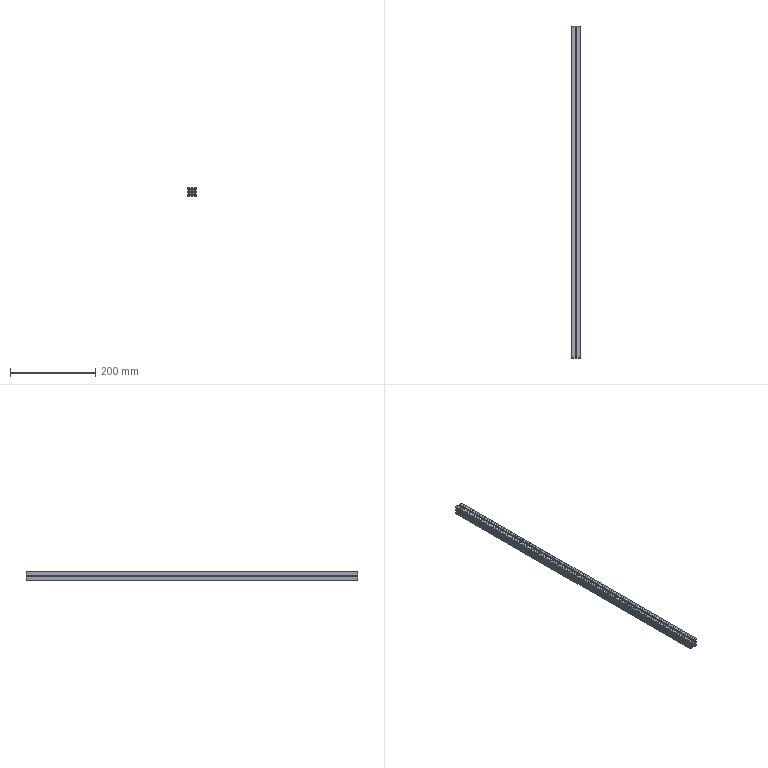Part | STEP file | 20 aluminium profile longitudinal 7 | 1 solid | 64 faces | box 20 x 778 x 20 mm | volume 138312 mm3 | plane 54 | cylinder 10 | commonest cylinder face diameters 3.3 x10